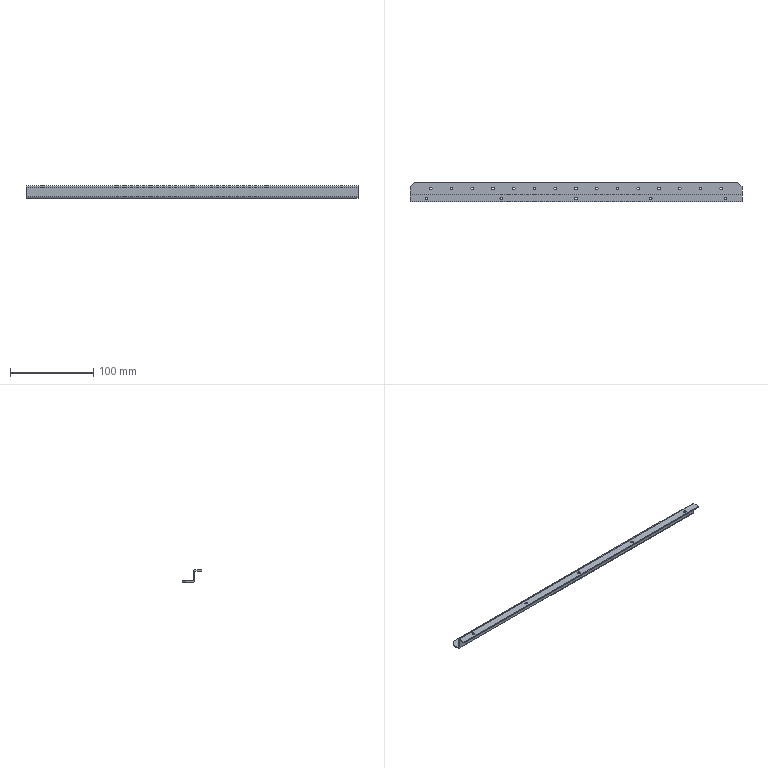Part | SolidWorks | features LPattern 4, EdgeFlange 2, ICE 2, Chamfer 1, FlatPattern 1, SMBaseFlange 1, SheetMetal 1 | 1 solid | 64 faces | box 400 x 23.5 x 15 mm | volume 21483 mm3 | cylinder 44 | plane 20 | commonest cylinder face diameters 3.2 x42 0.2 x2